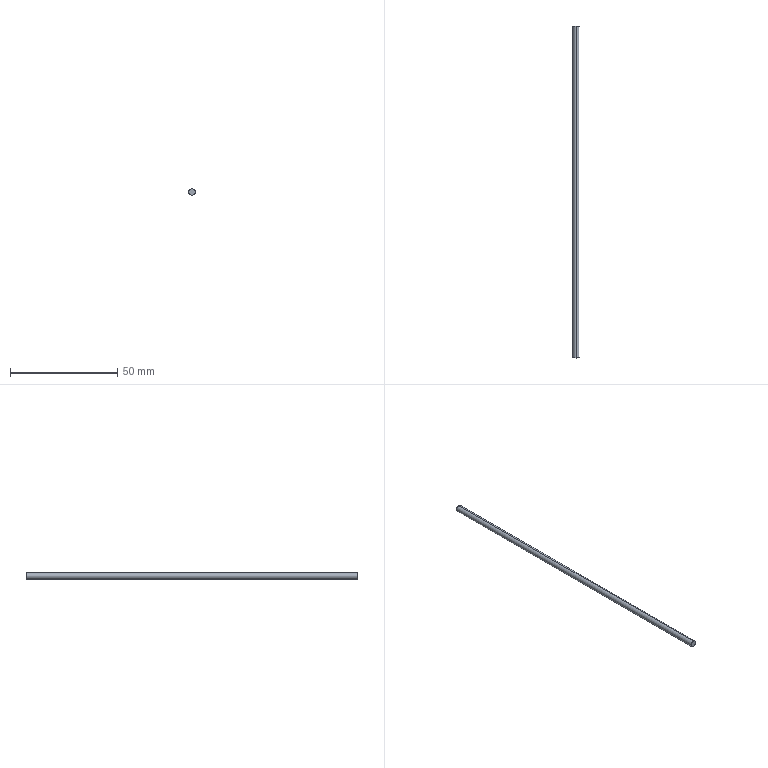Part | SolidWorks | features Extrusion 1 | 1 solid | 4 faces | box 3 x 155 x 3 mm | volume 1096 mm3 | cylinder 2 | plane 2 | commonest cylinder face diameters 3 x2
STEP:
#1=CARTESIAN_POINT('',(0.,155.,1.5));
#2=VERTEX_POINT('',#1);
#3=CARTESIAN_POINT('',(0.,155.,-1.5));
#4=VERTEX_POINT('',#3);
#5=CARTESIAN_POINT('',(0.,155.,0.));
#6=DIRECTION('',(0.,1.,0.));
#7=DIRECTION('',(0.,0.,1.));
#8=AXIS2_PLACEMENT_3D('',#5,#6,#7);
#9=CIRCLE('',#8,1.5);
#10=EDGE_CURVE('',#2,#4,#9,.T.);
#11=ORIENTED_EDGE('',*,*,#10,.F.);
#12=CARTESIAN_POINT('',(0.,0.,1.5));
#13=VERTEX_POINT('',#12);
#14=CARTESIAN_POINT('',(0.,155.,1.5));
#15=DIRECTION('',(0.,-1.,0.));
#16=VECTOR('',#15,1000.);
#17=LINE('',#14,#16);
#18=EDGE_CURVE('',#2,#13,#17,.T.);
#19=ORIENTED_EDGE('',*,*,#18,.T.);
#20=CARTESIAN_POINT('',(0.,0.,-1.5));
#21=VERTEX_POINT('',#20);
#22=CARTESIAN_POINT('',(0.,0.,0.));
#23=DIRECTION('',(0.,1.,0.));
#24=DIRECTION('',(0.,0.,1.));
#25=AXIS2_PLACEMENT_3D('',#22,#23,#24);
#26=CIRCLE('',#25,1.5);
#27=EDGE_CURVE('',#13,#21,#26,.T.);
#28=ORIENTED_EDGE('',*,*,#27,.T.);
#29=CARTESIAN_POINT('',(0.,155.,-1.5));
#30=DIRECTION('',(0.,-1.,0.));
#31=VECTOR('',#30,1000.);
#32=LINE('',#29,#31);
#33=EDGE_CURVE('',#4,#21,#32,.T.);
#34=ORIENTED_EDGE('',*,*,#33,.F.);
#35=EDGE_LOOP('',(#11,#19,#28,#34));
#36=FACE_OUTER_BOUND('',#35,.T.);
#37=CARTESIAN_POINT('',(0.,155.,0.));
#38=DIRECTION('',(0.,-1.,0.));
#39=DIRECTION('',(0.,0.,-1.));
#40=AXIS2_PLACEMENT_3D('',#37,#38,#39);
#41=CYLINDRICAL_SURFACE('',#40,1.5);
#42=ADVANCED_FACE('',(#36),#41,.T.);
#43=ORIENTED_EDGE('',*,*,#18,.F.);
#44=CARTESIAN_POINT('',(0.,155.,0.));
#45=DIRECTION('',(0.,1.,0.));
#46=DIRECTION('',(0.,0.,1.));
#47=AXIS2_PLACEMENT_3D('',#44,#45,#46);
#48=CIRCLE('',#47,1.5);
#49=EDGE_CURVE('',#4,#2,#48,.T.);
#50=ORIENTED_EDGE('',*,*,#49,.F.);
#51=ORIENTED_EDGE('',*,*,#33,.T.);
#52=CARTESIAN_POINT('',(0.,0.,0.));
#53=DIRECTION('',(0.,1.,0.));
#54=DIRECTION('',(0.,0.,1.));
#55=AXIS2_PLACEMENT_3D('',#52,#53,#54);
#56=CIRCLE('',#55,1.5);
#57=EDGE_CURVE('',#21,#13,#56,.T.);
#58=ORIENTED_EDGE('',*,*,#57,.T.);
#59=EDGE_LOOP('',(#43,#50,#51,#58));
#60=FACE_OUTER_BOUND('',#59,.T.);
#61=CARTESIAN_POINT('',(0.,155.,0.));
#62=DIRECTION('',(0.,-1.,0.));
#63=DIRECTION('',(0.,0.,-1.));
#64=AXIS2_PLACEMENT_3D('',#61,#62,#63);
#65=CYLINDRICAL_SURFACE('',#64,1.5);
#66=ADVANCED_FACE('',(#60),#65,.T.);
#67=ORIENTED_EDGE('',*,*,#49,.T.);
#68=ORIENTED_EDGE('',*,*,#10,.T.);
#69=EDGE_LOOP('',(#67,#68));
#70=FACE_OUTER_BOUND('',#69,.T.);
#71=CARTESIAN_POINT('',(0.,155.,0.));
#72=DIRECTION('',(0.,1.,0.));
#73=DIRECTION('',(0.,0.,1.));
#74=AXIS2_PLACEMENT_3D('',#71,#72,#73);
#75=PLANE('',#74);
#76=ADVANCED_FACE('',(#70),#75,.T.);
#77=ORIENTED_EDGE('',*,*,#57,.F.);
#78=ORIENTED_EDGE('',*,*,#27,.F.);
#79=EDGE_LOOP('',(#77,#78));
#80=FACE_OUTER_BOUND('',#79,.T.);
#81=CARTESIAN_POINT('',(0.,0.,0.));
#82=DIRECTION('',(0.,1.,0.));
#83=DIRECTION('',(0.,0.,1.));
#84=AXIS2_PLACEMENT_3D('',#81,#82,#83);
#85=PLANE('',#84);
#86=ADVANCED_FACE('',(#80),#85,.F.);
#87=CLOSED_SHELL('',(#42,#66,#76,#86));
#88=MANIFOLD_SOLID_BREP('',#87);
#89=CARTESIAN_POINT('',(0.,0.,0.));
#90=DIRECTION('',(0.,0.,1.));
#91=DIRECTION('',(1.,0.,0.));
#92=AXIS2_PLACEMENT_3D('',#89,#90,#91);
#93=(LENGTH_UNIT()NAMED_UNIT(*)SI_UNIT(.MILLI.,.METRE.));
#94=UNCERTAINTY_MEASURE_WITH_UNIT(LENGTH_MEASURE(0.00001),#93,'','');
#95=(NAMED_UNIT(*)PLANE_ANGLE_UNIT()SI_UNIT($,.RADIAN.));
#96=(NAMED_UNIT(*)SI_UNIT($,.STERADIAN.)SOLID_ANGLE_UNIT());
#97=(GEOMETRIC_REPRESENTATION_CONTEXT(3)GLOBAL_UNCERTAINTY_ASSIGNED_CONTEXT((#94))GLOBAL_UNIT_ASSIGNED_CONTEXT((#93,#95,#96))REPRESENTATION_CONTEXT('',''));
#98=ADVANCED_BREP_SHAPE_REPRESENTATION('',(#88,#92),#97);